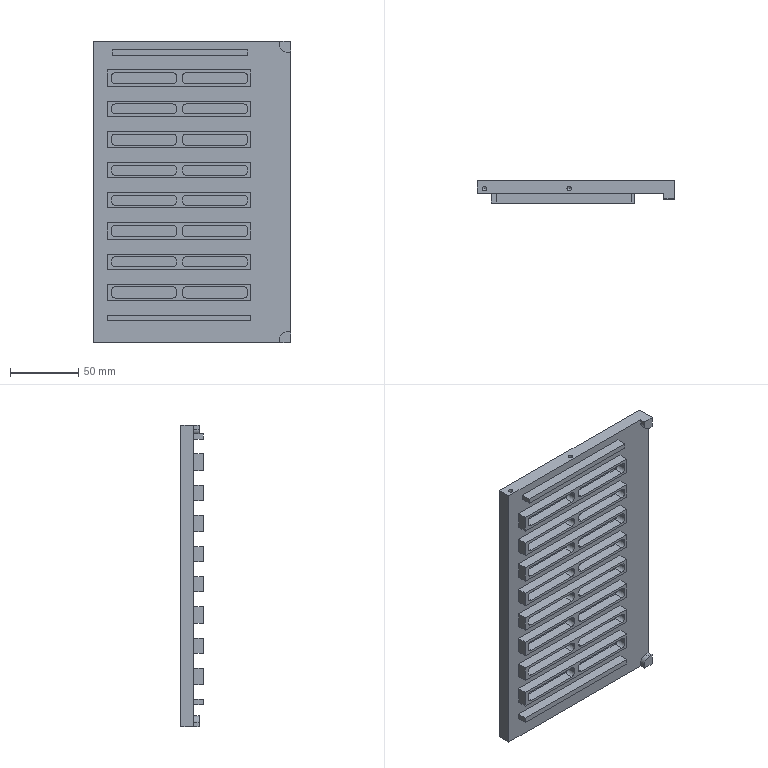NC program | NX | posted with a generic post | part box 144.5 x 16.5 x 221 mm
Lines 1 to 24 of 8751:
N10 G17 G21 G94 G90
(FLOOR_WALL , TOOL : D63面刀)
N12 T01 M6
N14 G53
N16 G17 G0 G90 X152. Y-63.25 B0. C0. S3500 M3
N18 G43 Z20. H1
N20 Z3.1
N22 G94 G1 Z0.1 F1000.
N24 X149.
N26 X-149.
N28 Y-24.233
N30 X149.
N32 Y14.783
N34 X-149.
N36 Y53.8
N38 X149.
N40 X152.
N42 Z3.1
N44 G0 Z20.
N46 M5